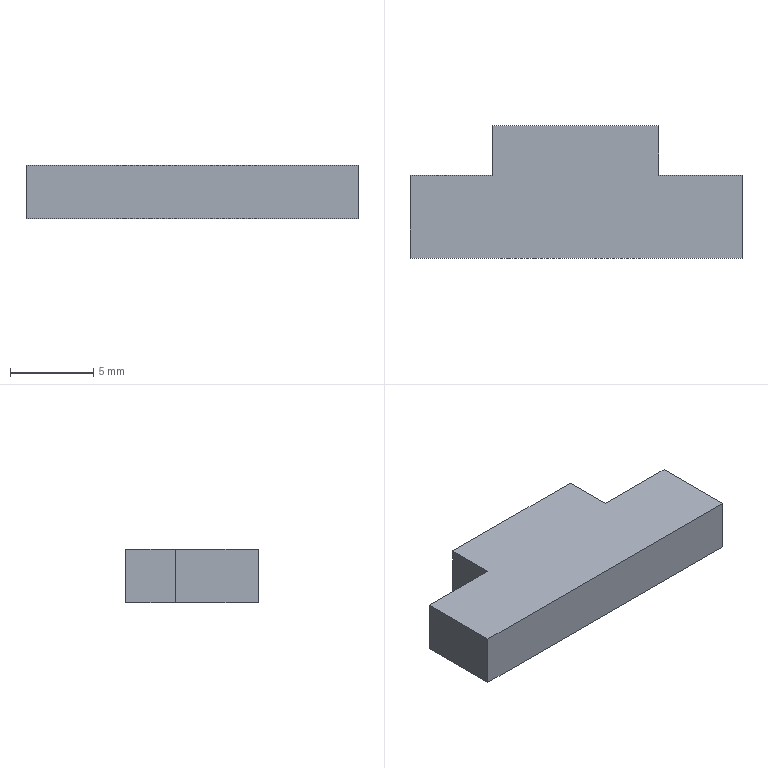Part | SolidWorks | features FlatPattern 1, SMBaseFlange 1, SheetMetal 1 | 1 solid | 10 faces | box 20 x 8 x 3.2 mm | volume 416 mm3 | plane 10
STEP:
#1=CARTESIAN_POINT('',(113.5,0.,0.));
#2=VERTEX_POINT('',#1);
#3=CARTESIAN_POINT('',(108.5,0.,0.));
#4=VERTEX_POINT('',#3);
#5=CARTESIAN_POINT('',(108.5,0.,0.));
#6=DIRECTION('',(-1.,0.,0.));
#7=VECTOR('',#6,1000.);
#8=LINE('',#5,#7);
#9=EDGE_CURVE('',#2,#4,#8,.T.);
#10=ORIENTED_EDGE('',*,*,#9,.T.);
#11=CARTESIAN_POINT('',(108.5,0.,3.2));
#12=VERTEX_POINT('',#11);
#13=CARTESIAN_POINT('',(108.5,0.,3.2));
#14=DIRECTION('',(0.,0.,-1.));
#15=VECTOR('',#14,1000.);
#16=LINE('',#13,#15);
#17=EDGE_CURVE('',#12,#4,#16,.T.);
#18=ORIENTED_EDGE('',*,*,#17,.F.);
#19=CARTESIAN_POINT('',(113.5,0.,3.2));
#20=VERTEX_POINT('',#19);
#21=CARTESIAN_POINT('',(108.5,0.,3.2));
#22=DIRECTION('',(-1.,0.,0.));
#23=VECTOR('',#22,1000.);
#24=LINE('',#21,#23);
#25=EDGE_CURVE('',#20,#12,#24,.T.);
#26=ORIENTED_EDGE('',*,*,#25,.F.);
#27=CARTESIAN_POINT('',(113.5,0.,3.2));
#28=DIRECTION('',(0.,0.,-1.));
#29=VECTOR('',#28,1000.);
#30=LINE('',#27,#29);
#31=EDGE_CURVE('',#20,#2,#30,.T.);
#32=ORIENTED_EDGE('',*,*,#31,.T.);
#33=EDGE_LOOP('',(#10,#18,#26,#32));
#34=FACE_OUTER_BOUND('',#33,.T.);
#35=CARTESIAN_POINT('',(108.5,0.,3.2));
#36=DIRECTION('',(0.,-1.,0.));
#37=DIRECTION('',(1.,0.,0.));
#38=AXIS2_PLACEMENT_3D('',#35,#36,#37);
#39=PLANE('',#38);
#40=ADVANCED_FACE('',(#34),#39,.F.);
#41=CARTESIAN_POINT('',(108.5,-5.,0.));
#42=VERTEX_POINT('',#41);
#43=CARTESIAN_POINT('',(108.5,-5.,0.));
#44=DIRECTION('',(0.,-1.,0.));
#45=VECTOR('',#44,1000.);
#46=LINE('',#43,#45);
#47=EDGE_CURVE('',#4,#42,#46,.T.);
#48=ORIENTED_EDGE('',*,*,#47,.T.);
#49=CARTESIAN_POINT('',(108.5,-5.,3.2));
#50=VERTEX_POINT('',#49);
#51=CARTESIAN_POINT('',(108.5,-5.,3.2));
#52=DIRECTION('',(0.,0.,-1.));
#53=VECTOR('',#52,1000.);
#54=LINE('',#51,#53);
#55=EDGE_CURVE('',#50,#42,#54,.T.);
#56=ORIENTED_EDGE('',*,*,#55,.F.);
#57=CARTESIAN_POINT('',(108.5,-5.,3.2));
#58=DIRECTION('',(0.,-1.,0.));
#59=VECTOR('',#58,1000.);
#60=LINE('',#57,#59);
#61=EDGE_CURVE('',#12,#50,#60,.T.);
#62=ORIENTED_EDGE('',*,*,#61,.F.);
#63=ORIENTED_EDGE('',*,*,#17,.T.);
#64=EDGE_LOOP('',(#48,#56,#62,#63));
#65=FACE_OUTER_BOUND('',#64,.T.);
#66=CARTESIAN_POINT('',(108.5,-5.,3.2));
#67=DIRECTION('',(1.,0.,0.));
#68=DIRECTION('',(0.,0.,-1.));
#69=AXIS2_PLACEMENT_3D('',#66,#67,#68);
#70=PLANE('',#69);
#71=ADVANCED_FACE('',(#65),#70,.F.);
#72=CARTESIAN_POINT('',(128.5,-5.,0.));
#73=VERTEX_POINT('',#72);
#74=CARTESIAN_POINT('',(128.5,-5.,0.));
#75=DIRECTION('',(1.,0.,0.));
#76=VECTOR('',#75,1000.);
#77=LINE('',#74,#76);
#78=EDGE_CURVE('',#42,#73,#77,.T.);
#79=ORIENTED_EDGE('',*,*,#78,.T.);
#80=CARTESIAN_POINT('',(128.5,-5.,3.2));
#81=VERTEX_POINT('',#80);
#82=CARTESIAN_POINT('',(128.5,-5.,3.2));
#83=DIRECTION('',(0.,0.,-1.));
#84=VECTOR('',#83,1000.);
#85=LINE('',#82,#84);
#86=EDGE_CURVE('',#81,#73,#85,.T.);
#87=ORIENTED_EDGE('',*,*,#86,.F.);
#88=CARTESIAN_POINT('',(128.5,-5.,3.2));
#89=DIRECTION('',(1.,0.,0.));
#90=VECTOR('',#89,1000.);
#91=LINE('',#88,#90);
#92=EDGE_CURVE('',#50,#81,#91,.T.);
#93=ORIENTED_EDGE('',*,*,#92,.F.);
#94=ORIENTED_EDGE('',*,*,#55,.T.);
#95=EDGE_LOOP('',(#79,#87,#93,#94));
#96=FACE_OUTER_BOUND('',#95,.T.);
#97=CARTESIAN_POINT('',(128.5,-5.,3.2));
#98=DIRECTION('',(0.,1.,0.));
#99=DIRECTION('',(-1.,0.,0.));
#100=AXIS2_PLACEMENT_3D('',#97,#98,#99);
#101=PLANE('',#100);
#102=ADVANCED_FACE('',(#96),#101,.F.);
#103=CARTESIAN_POINT('',(128.5,0.,0.));
#104=VERTEX_POINT('',#103);
#105=CARTESIAN_POINT('',(128.5,0.,0.));
#106=DIRECTION('',(0.,1.,0.));
#107=VECTOR('',#106,1000.);
#108=LINE('',#105,#107);
#109=EDGE_CURVE('',#73,#104,#108,.T.);
#110=ORIENTED_EDGE('',*,*,#109,.T.);
#111=CARTESIAN_POINT('',(128.5,0.,3.2));
#112=VERTEX_POINT('',#111);
#113=CARTESIAN_POINT('',(128.5,0.,3.2));
#114=DIRECTION('',(0.,0.,-1.));
#115=VECTOR('',#114,1000.);
#116=LINE('',#113,#115);
#117=EDGE_CURVE('',#112,#104,#116,.T.);
#118=ORIENTED_EDGE('',*,*,#117,.F.);
#119=CARTESIAN_POINT('',(128.5,0.,3.2));
#120=DIRECTION('',(0.,1.,0.));
#121=VECTOR('',#120,1000.);
#122=LINE('',#119,#121);
#123=EDGE_CURVE('',#81,#112,#122,.T.);
#124=ORIENTED_EDGE('',*,*,#123,.F.);
#125=ORIENTED_EDGE('',*,*,#86,.T.);
#126=EDGE_LOOP('',(#110,#118,#124,#125));
#127=FACE_OUTER_BOUND('',#126,.T.);
#128=CARTESIAN_POINT('',(128.5,0.,3.2));
#129=DIRECTION('',(-1.,0.,0.));
#130=DIRECTION('',(0.,0.,1.));
#131=AXIS2_PLACEMENT_3D('',#128,#129,#130);
#132=PLANE('',#131);
#133=ADVANCED_FACE('',(#127),#132,.F.);
#134=CARTESIAN_POINT('',(123.5,0.,0.));
#135=VERTEX_POINT('',#134);
#136=CARTESIAN_POINT('',(123.5,0.,0.));
#137=DIRECTION('',(-1.,0.,0.));
#138=VECTOR('',#137,1000.);
#139=LINE('',#136,#138);
#140=EDGE_CURVE('',#104,#135,#139,.T.);
#141=ORIENTED_EDGE('',*,*,#140,.T.);
#142=CARTESIAN_POINT('',(123.5,0.,3.2));
#143=VERTEX_POINT('',#142);
#144=CARTESIAN_POINT('',(123.5,0.,3.2));
#145=DIRECTION('',(0.,0.,-1.));
#146=VECTOR('',#145,1000.);
#147=LINE('',#144,#146);
#148=EDGE_CURVE('',#143,#135,#147,.T.);
#149=ORIENTED_EDGE('',*,*,#148,.F.);
#150=CARTESIAN_POINT('',(123.5,0.,3.2));
#151=DIRECTION('',(-1.,0.,0.));
#152=VECTOR('',#151,1000.);
#153=LINE('',#150,#152);
#154=EDGE_CURVE('',#112,#143,#153,.T.);
#155=ORIENTED_EDGE('',*,*,#154,.F.);
#156=ORIENTED_EDGE('',*,*,#117,.T.);
#157=EDGE_LOOP('',(#141,#149,#155,#156));
#158=FACE_OUTER_BOUND('',#157,.T.);
#159=CARTESIAN_POINT('',(123.5,0.,3.2));
#160=DIRECTION('',(0.,-1.,0.));
#161=DIRECTION('',(0.,0.,-1.));
#162=AXIS2_PLACEMENT_3D('',#159,#160,#161);
#163=PLANE('',#162);
#164=ADVANCED_FACE('',(#158),#163,.F.);
#165=CARTESIAN_POINT('',(123.5,3.,0.));
#166=VERTEX_POINT('',#165);
#167=CARTESIAN_POINT('',(123.5,3.,0.));
#168=DIRECTION('',(0.,1.,0.));
#169=VECTOR('',#168,1000.);
#170=LINE('',#167,#169);
#171=EDGE_CURVE('',#135,#166,#170,.T.);
#172=ORIENTED_EDGE('',*,*,#171,.T.);
#173=CARTESIAN_POINT('',(123.5,3.,3.2));
#174=VERTEX_POINT('',#173);
#175=CARTESIAN_POINT('',(123.5,3.,3.2));
#176=DIRECTION('',(0.,0.,-1.));
#177=VECTOR('',#176,1000.);
#178=LINE('',#175,#177);
#179=EDGE_CURVE('',#174,#166,#178,.T.);
#180=ORIENTED_EDGE('',*,*,#179,.F.);
#181=CARTESIAN_POINT('',(123.5,3.,3.2));
#182=DIRECTION('',(0.,1.,0.));
#183=VECTOR('',#182,1000.);
#184=LINE('',#181,#183);
#185=EDGE_CURVE('',#143,#174,#184,.T.);
#186=ORIENTED_EDGE('',*,*,#185,.F.);
#187=ORIENTED_EDGE('',*,*,#148,.T.);
#188=EDGE_LOOP('',(#172,#180,#186,#187));
#189=FACE_OUTER_BOUND('',#188,.T.);
#190=CARTESIAN_POINT('',(123.5,3.,3.2));
#191=DIRECTION('',(-1.,0.,0.));
#192=DIRECTION('',(0.,0.,1.));
#193=AXIS2_PLACEMENT_3D('',#190,#191,#192);
#194=PLANE('',#193);
#195=ADVANCED_FACE('',(#189),#194,.F.);
#196=CARTESIAN_POINT('',(113.5,3.,0.));
#197=VERTEX_POINT('',#196);
#198=CARTESIAN_POINT('',(113.5,3.,0.));
#199=DIRECTION('',(-1.,0.,0.));
#200=VECTOR('',#199,1000.);
#201=LINE('',#198,#200);
#202=EDGE_CURVE('',#166,#197,#201,.T.);
#203=ORIENTED_EDGE('',*,*,#202,.T.);
#204=CARTESIAN_POINT('',(113.5,3.,3.2));
#205=VERTEX_POINT('',#204);
#206=CARTESIAN_POINT('',(113.5,3.,3.2));
#207=DIRECTION('',(0.,0.,-1.));
#208=VECTOR('',#207,1000.);
#209=LINE('',#206,#208);
#210=EDGE_CURVE('',#205,#197,#209,.T.);
#211=ORIENTED_EDGE('',*,*,#210,.F.);
#212=CARTESIAN_POINT('',(113.5,3.,3.2));
#213=DIRECTION('',(-1.,0.,0.));
#214=VECTOR('',#213,1000.);
#215=LINE('',#212,#214);
#216=EDGE_CURVE('',#174,#205,#215,.T.);
#217=ORIENTED_EDGE('',*,*,#216,.F.);
#218=ORIENTED_EDGE('',*,*,#179,.T.);
#219=EDGE_LOOP('',(#203,#211,#217,#218));
#220=FACE_OUTER_BOUND('',#219,.T.);
#221=CARTESIAN_POINT('',(113.5,3.,3.2));
#222=DIRECTION('',(0.,-1.,0.));
#223=DIRECTION('',(0.,0.,-1.));
#224=AXIS2_PLACEMENT_3D('',#221,#222,#223);
#225=PLANE('',#224);
#226=ADVANCED_FACE('',(#220),#225,.F.);
#227=CARTESIAN_POINT('',(113.5,0.,0.));
#228=DIRECTION('',(0.,-1.,0.));
#229=VECTOR('',#228,1000.);
#230=LINE('',#227,#229);
#231=EDGE_CURVE('',#197,#2,#230,.T.);
#232=ORIENTED_EDGE('',*,*,#231,.T.);
#233=ORIENTED_EDGE('',*,*,#31,.F.);
#234=CARTESIAN_POINT('',(113.5,0.,3.2));
#235=DIRECTION('',(0.,-1.,0.));
#236=VECTOR('',#235,1000.);
#237=LINE('',#234,#236);
#238=EDGE_CURVE('',#205,#20,#237,.T.);
#239=ORIENTED_EDGE('',*,*,#238,.F.);
#240=ORIENTED_EDGE('',*,*,#210,.T.);
#241=EDGE_LOOP('',(#232,#233,#239,#240));
#242=FACE_OUTER_BOUND('',#241,.T.);
#243=CARTESIAN_POINT('',(113.5,0.,3.2));
#244=DIRECTION('',(1.,0.,0.));
#245=DIRECTION('',(0.,0.,-1.));
#246=AXIS2_PLACEMENT_3D('',#243,#244,#245);
#247=PLANE('',#246);
#248=ADVANCED_FACE('',(#242),#247,.F.);
#249=ORIENTED_EDGE('',*,*,#25,.T.);
#250=ORIENTED_EDGE('',*,*,#61,.T.);
#251=ORIENTED_EDGE('',*,*,#92,.T.);
#252=ORIENTED_EDGE('',*,*,#123,.T.);
#253=ORIENTED_EDGE('',*,*,#154,.T.);
#254=ORIENTED_EDGE('',*,*,#185,.T.);
#255=ORIENTED_EDGE('',*,*,#216,.T.);
#256=ORIENTED_EDGE('',*,*,#238,.T.);
#257=EDGE_LOOP('',(#249,#250,#251,#252,#253,#254,#255,#256));
#258=FACE_OUTER_BOUND('',#257,.T.);
#259=CARTESIAN_POINT('',(0.,0.,3.2));
#260=DIRECTION('',(0.,0.,1.));
#261=DIRECTION('',(1.,0.,0.));
#262=AXIS2_PLACEMENT_3D('',#259,#260,#261);
#263=PLANE('',#262);
#264=ADVANCED_FACE('',(#258),#263,.T.);
#265=ORIENTED_EDGE('',*,*,#9,.F.);
#266=ORIENTED_EDGE('',*,*,#231,.F.);
#267=ORIENTED_EDGE('',*,*,#202,.F.);
#268=ORIENTED_EDGE('',*,*,#171,.F.);
#269=ORIENTED_EDGE('',*,*,#140,.F.);
#270=ORIENTED_EDGE('',*,*,#109,.F.);
#271=ORIENTED_EDGE('',*,*,#78,.F.);
#272=ORIENTED_EDGE('',*,*,#47,.F.);
#273=EDGE_LOOP('',(#265,#266,#267,#268,#269,#270,#271,#272));
#274=FACE_OUTER_BOUND('',#273,.T.);
#275=CARTESIAN_POINT('',(0.,0.,0.));
#276=DIRECTION('',(0.,0.,1.));
#277=DIRECTION('',(1.,0.,0.));
#278=AXIS2_PLACEMENT_3D('',#275,#276,#277);
#279=PLANE('',#278);
#280=ADVANCED_FACE('',(#274),#279,.F.);
#281=CLOSED_SHELL('',(#40,#71,#102,#133,#164,#195,#226,#248,#264,#280));
#282=MANIFOLD_SOLID_BREP('',#281);
#283=CARTESIAN_POINT('',(0.,0.,0.));
#284=DIRECTION('',(0.,0.,1.));
#285=DIRECTION('',(1.,0.,0.));
#286=AXIS2_PLACEMENT_3D('',#283,#284,#285);
#287=(LENGTH_UNIT()NAMED_UNIT(*)SI_UNIT(.MILLI.,.METRE.));
#288=UNCERTAINTY_MEASURE_WITH_UNIT(LENGTH_MEASURE(0.00001),#287,'','');
#289=(NAMED_UNIT(*)PLANE_ANGLE_UNIT()SI_UNIT($,.RADIAN.));
#290=(NAMED_UNIT(*)SI_UNIT($,.STERADIAN.)SOLID_ANGLE_UNIT());
#291=(GEOMETRIC_REPRESENTATION_CONTEXT(3)GLOBAL_UNCERTAINTY_ASSIGNED_CONTEXT((#288))GLOBAL_UNIT_ASSIGNED_CONTEXT((#287,#289,#290))REPRESENTATION_CONTEXT('',''));
#292=ADVANCED_BREP_SHAPE_REPRESENTATION('',(#282,#286),#291);